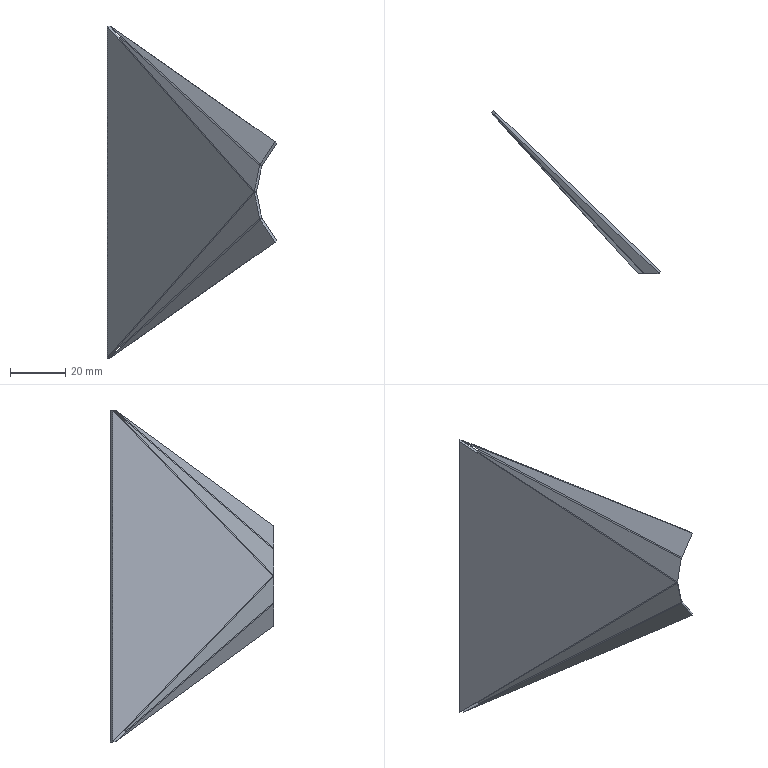Part | STEP file | JBJ-P-1003-09 | 1 solid | 42 faces | box 61.208 x 58.943 x 119.791 mm | volume 7806 mm3 | plane 32 | cylinder 8 | spline 2 | commonest cylinder face diameters 2 x4 4.4 x4
STEP:
#1=CARTESIAN_POINT('',(-30.002,-185.39,-9.425));
#2=VERTEX_POINT('',#1);
#3=CARTESIAN_POINT('',(-30.795,-186.277,-9.583));
#4=VERTEX_POINT('',#3);
#5=CARTESIAN_POINT('',(-30.002,-185.39,-9.425));
#6=DIRECTION('',(-0.6604,-0.7393,-0.1314));
#7=VECTOR('',#6,1000.);
#8=LINE('',#5,#7);
#9=EDGE_CURVE('',#2,#4,#8,.T.);
#10=ORIENTED_EDGE('',*,*,#9,.F.);
#11=CARTESIAN_POINT('',(-31.859,-185.39,-0.09366));
#12=VERTEX_POINT('',#11);
#13=CARTESIAN_POINT('',(-31.877,-185.39,0.));
#14=DIRECTION('',(0.1951,0.,-0.9808));
#15=VECTOR('',#14,1000.);
#16=LINE('',#13,#15);
#17=EDGE_CURVE('',#12,#2,#16,.T.);
#18=ORIENTED_EDGE('',*,*,#17,.F.);
#19=CARTESIAN_POINT('',(-32.651,-186.277,-0.2513));
#20=VERTEX_POINT('',#19);
#21=CARTESIAN_POINT('',(-31.859,-185.39,-0.09366));
#22=DIRECTION('',(-0.6604,-0.7393,-0.1314));
#23=VECTOR('',#22,1000.);
#24=LINE('',#21,#23);
#25=EDGE_CURVE('',#12,#20,#24,.T.);
#26=ORIENTED_EDGE('',*,*,#25,.T.);
#27=CARTESIAN_POINT('',(-32.67,-186.277,-0.1576));
#28=DIRECTION('',(0.1951,0.,-0.9808));
#29=VECTOR('',#28,1000.);
#30=LINE('',#27,#29);
#31=EDGE_CURVE('',#20,#4,#30,.T.);
#32=ORIENTED_EDGE('',*,*,#31,.T.);
#33=EDGE_LOOP('',(#10,#18,#26,#32));
#34=FACE_OUTER_BOUND('',#33,.T.);
#35=CARTESIAN_POINT('',(-31.877,-185.39,0.));
#36=DIRECTION('',(0.7251,-0.6733,0.1442));
#37=DIRECTION('',(0.1951,0.,-0.9808));
#38=AXIS2_PLACEMENT_3D('',#35,#36,#37);
#39=PLANE('',#38);
#40=ADVANCED_FACE('',(#34),#39,.T.);
#41=ORIENTED_EDGE('',*,*,#25,.F.);
#42=CARTESIAN_POINT('',(-32.113,-185.112,-0.3814));
#43=VERTEX_POINT('',#42);
#44=CARTESIAN_POINT('',(-80.984,-131.63,-55.707));
#45=DIRECTION('',(-0.5361,0.5867,-0.6069));
#46=VECTOR('',#45,1000.);
#47=LINE('',#44,#46);
#48=EDGE_CURVE('',#12,#43,#47,.T.);
#49=ORIENTED_EDGE('',*,*,#48,.T.);
#50=CARTESIAN_POINT('',(-32.905,-185.999,-0.539));
#51=VERTEX_POINT('',#50);
#52=CARTESIAN_POINT('',(-32.113,-185.112,-0.3814));
#53=DIRECTION('',(-0.6604,-0.7393,-0.1314));
#54=VECTOR('',#53,1000.);
#55=LINE('',#52,#54);
#56=EDGE_CURVE('',#43,#51,#55,.T.);
#57=ORIENTED_EDGE('',*,*,#56,.T.);
#58=CARTESIAN_POINT('',(-81.776,-132.518,-55.865));
#59=DIRECTION('',(-0.5361,0.5867,-0.6069));
#60=VECTOR('',#59,1000.);
#61=LINE('',#58,#60);
#62=EDGE_CURVE('',#20,#51,#61,.T.);
#63=ORIENTED_EDGE('',*,*,#62,.F.);
#64=EDGE_LOOP('',(#41,#49,#57,#63));
#65=FACE_OUTER_BOUND('',#64,.T.);
#66=CARTESIAN_POINT('',(-80.984,-131.63,-55.707));
#67=DIRECTION('',(0.5258,-0.3304,-0.7838));
#68=DIRECTION('',(-0.5361,0.5867,-0.6069));
#69=AXIS2_PLACEMENT_3D('',#66,#67,#68);
#70=PLANE('',#69);
#71=ADVANCED_FACE('',(#65),#70,.F.);
#72=ORIENTED_EDGE('',*,*,#56,.F.);
#73=CARTESIAN_POINT('',(-32.19,-185.047,-0.25));
#74=VERTEX_POINT('',#73);
#75=CARTESIAN_POINT('',(-31.452,-184.373,-0.25));
#76=DIRECTION('',(-0.5361,0.5867,-0.6069));
#77=DIRECTION('',(0.,0.719,0.695));
#78=AXIS2_PLACEMENT_3D('',#75,#76,#77);
#79=CIRCLE('',#78,1.);
#80=EDGE_CURVE('',#43,#74,#79,.T.);
#81=ORIENTED_EDGE('',*,*,#80,.T.);
#82=CARTESIAN_POINT('',(-33.076,-185.857,-0.25));
#83=VERTEX_POINT('',#82);
#84=CARTESIAN_POINT('',(-32.19,-185.047,-0.25));
#85=DIRECTION('',(-0.7382,-0.6746,0.));
#86=VECTOR('',#85,1000.);
#87=LINE('',#84,#86);
#88=EDGE_CURVE('',#74,#83,#87,.T.);
#89=ORIENTED_EDGE('',*,*,#88,.T.);
#90=CARTESIAN_POINT('',(-31.452,-184.373,-0.25));
#91=DIRECTION('',(-0.5361,0.5867,-0.6069));
#92=DIRECTION('',(0.,-0.719,-0.695));
#93=AXIS2_PLACEMENT_3D('',#90,#91,#92);
#94=CIRCLE('',#93,2.2);
#95=EDGE_CURVE('',#51,#83,#94,.T.);
#96=ORIENTED_EDGE('',*,*,#95,.F.);
#97=EDGE_LOOP('',(#72,#81,#89,#96));
#98=FACE_OUTER_BOUND('',#97,.T.);
#99=CARTESIAN_POINT('',(-31.452,-184.373,-0.25));
#100=DIRECTION('',(0.5361,-0.5867,0.6069));
#101=DIRECTION('',(0.,-0.719,-0.695));
#102=AXIS2_PLACEMENT_3D('',#99,#100,#101);
#103=PLANE('',#102);
#104=ADVANCED_FACE('',(#98),#103,.T.);
#105=ORIENTED_EDGE('',*,*,#88,.F.);
#106=CARTESIAN_POINT('',(-32.19,-185.047,0.25));
#107=VERTEX_POINT('',#106);
#108=CARTESIAN_POINT('',(-32.19,-185.047,0.));
#109=DIRECTION('',(0.,0.,-1.));
#110=VECTOR('',#109,1000.);
#111=LINE('',#108,#110);
#112=EDGE_CURVE('',#107,#74,#111,.T.);
#113=ORIENTED_EDGE('',*,*,#112,.F.);
#114=CARTESIAN_POINT('',(-33.076,-185.857,0.25));
#115=VERTEX_POINT('',#114);
#116=CARTESIAN_POINT('',(-32.19,-185.047,0.25));
#117=DIRECTION('',(-0.7382,-0.6746,0.));
#118=VECTOR('',#117,1000.);
#119=LINE('',#116,#118);
#120=EDGE_CURVE('',#107,#115,#119,.T.);
#121=ORIENTED_EDGE('',*,*,#120,.T.);
#122=CARTESIAN_POINT('',(-33.076,-185.857,0.));
#123=DIRECTION('',(0.,0.,-1.));
#124=VECTOR('',#123,1000.);
#125=LINE('',#122,#124);
#126=EDGE_CURVE('',#115,#83,#125,.T.);
#127=ORIENTED_EDGE('',*,*,#126,.T.);
#128=EDGE_LOOP('',(#105,#113,#121,#127));
#129=FACE_OUTER_BOUND('',#128,.T.);
#130=CARTESIAN_POINT('',(-32.19,-185.047,0.));
#131=DIRECTION('',(0.6746,-0.7382,0.));
#132=DIRECTION('',(0.,0.,-1.));
#133=AXIS2_PLACEMENT_3D('',#130,#131,#132);
#134=PLANE('',#133);
#135=ADVANCED_FACE('',(#129),#134,.T.);
#136=ORIENTED_EDGE('',*,*,#120,.F.);
#137=CARTESIAN_POINT('',(-32.113,-185.112,0.3814));
#138=VERTEX_POINT('',#137);
#139=CARTESIAN_POINT('',(-31.452,-184.373,0.25));
#140=DIRECTION('',(-0.5361,0.5867,0.6069));
#141=DIRECTION('',(0.,-0.719,0.695));
#142=AXIS2_PLACEMENT_3D('',#139,#140,#141);
#143=CIRCLE('',#142,1.);
#144=EDGE_CURVE('',#107,#138,#143,.T.);
#145=ORIENTED_EDGE('',*,*,#144,.T.);
#146=CARTESIAN_POINT('',(-32.905,-185.999,0.539));
#147=VERTEX_POINT('',#146);
#148=CARTESIAN_POINT('',(-32.113,-185.112,0.3814));
#149=DIRECTION('',(-0.6604,-0.7393,0.1314));
#150=VECTOR('',#149,1000.);
#151=LINE('',#148,#150);
#152=EDGE_CURVE('',#138,#147,#151,.T.);
#153=ORIENTED_EDGE('',*,*,#152,.T.);
#154=CARTESIAN_POINT('',(-31.452,-184.373,0.25));
#155=DIRECTION('',(-0.5361,0.5867,0.6069));
#156=DIRECTION('',(0.,0.719,-0.695));
#157=AXIS2_PLACEMENT_3D('',#154,#155,#156);
#158=CIRCLE('',#157,2.2);
#159=EDGE_CURVE('',#115,#147,#158,.T.);
#160=ORIENTED_EDGE('',*,*,#159,.F.);
#161=EDGE_LOOP('',(#136,#145,#153,#160));
#162=FACE_OUTER_BOUND('',#161,.T.);
#163=CARTESIAN_POINT('',(-31.452,-184.373,0.25));
#164=DIRECTION('',(0.5361,-0.5867,-0.6069));
#165=DIRECTION('',(0.,0.719,-0.695));
#166=AXIS2_PLACEMENT_3D('',#163,#164,#165);
#167=PLANE('',#166);
#168=ADVANCED_FACE('',(#162),#167,.T.);
#169=ORIENTED_EDGE('',*,*,#152,.F.);
#170=CARTESIAN_POINT('',(-31.859,-185.39,0.09367));
#171=VERTEX_POINT('',#170);
#172=CARTESIAN_POINT('',(-80.984,-131.63,55.707));
#173=DIRECTION('',(0.5361,-0.5867,-0.6069));
#174=VECTOR('',#173,1000.);
#175=LINE('',#172,#174);
#176=EDGE_CURVE('',#138,#171,#175,.T.);
#177=ORIENTED_EDGE('',*,*,#176,.T.);
#178=CARTESIAN_POINT('',(-32.651,-186.277,0.2513));
#179=VERTEX_POINT('',#178);
#180=CARTESIAN_POINT('',(-31.859,-185.39,0.09367));
#181=DIRECTION('',(-0.6604,-0.7393,0.1314));
#182=VECTOR('',#181,1000.);
#183=LINE('',#180,#182);
#184=EDGE_CURVE('',#171,#179,#183,.T.);
#185=ORIENTED_EDGE('',*,*,#184,.T.);
#186=CARTESIAN_POINT('',(-81.776,-132.518,55.865));
#187=DIRECTION('',(0.5361,-0.5867,-0.6069));
#188=VECTOR('',#187,1000.);
#189=LINE('',#186,#188);
#190=EDGE_CURVE('',#147,#179,#189,.T.);
#191=ORIENTED_EDGE('',*,*,#190,.F.);
#192=EDGE_LOOP('',(#169,#177,#185,#191));
#193=FACE_OUTER_BOUND('',#192,.T.);
#194=CARTESIAN_POINT('',(-80.984,-131.63,55.707));
#195=DIRECTION('',(-0.5258,0.3304,-0.7838));
#196=DIRECTION('',(0.5361,-0.5867,-0.6069));
#197=AXIS2_PLACEMENT_3D('',#194,#195,#196);
#198=PLANE('',#197);
#199=ADVANCED_FACE('',(#193),#198,.T.);
#200=ORIENTED_EDGE('',*,*,#184,.F.);
#201=CARTESIAN_POINT('',(-30.002,-185.39,9.425));
#202=VERTEX_POINT('',#201);
#203=CARTESIAN_POINT('',(-29.974,-185.39,9.567));
#204=DIRECTION('',(-0.1951,0.,-0.9808));
#205=VECTOR('',#204,1000.);
#206=LINE('',#203,#205);
#207=EDGE_CURVE('',#202,#171,#206,.T.);
#208=ORIENTED_EDGE('',*,*,#207,.F.);
#209=CARTESIAN_POINT('',(-30.795,-186.277,9.583));
#210=VERTEX_POINT('',#209);
#211=CARTESIAN_POINT('',(-30.002,-185.39,9.425));
#212=DIRECTION('',(-0.6604,-0.7393,0.1314));
#213=VECTOR('',#212,1000.);
#214=LINE('',#211,#213);
#215=EDGE_CURVE('',#202,#210,#214,.T.);
#216=ORIENTED_EDGE('',*,*,#215,.T.);
#217=CARTESIAN_POINT('',(-30.766,-186.277,9.725));
#218=DIRECTION('',(-0.1951,0.,-0.9808));
#219=VECTOR('',#218,1000.);
#220=LINE('',#217,#219);
#221=EDGE_CURVE('',#210,#179,#220,.T.);
#222=ORIENTED_EDGE('',*,*,#221,.T.);
#223=EDGE_LOOP('',(#200,#208,#216,#222));
#224=FACE_OUTER_BOUND('',#223,.T.);
#225=CARTESIAN_POINT('',(-29.974,-185.39,9.567));
#226=DIRECTION('',(-0.7251,0.6733,0.1442));
#227=DIRECTION('',(-0.1951,0.,-0.9808));
#228=AXIS2_PLACEMENT_3D('',#225,#226,#227);
#229=PLANE('',#228);
#230=ADVANCED_FACE('',(#224),#229,.F.);
#231=ORIENTED_EDGE('',*,*,#215,.F.);
#232=CARTESIAN_POINT('',(-29.9,-185.39,9.678));
#233=VERTEX_POINT('',#232);
#234=CARTESIAN_POINT('',(-30.002,-185.39,9.425));
#235=CARTESIAN_POINT('',(-29.983,-185.39,9.52));
#236=CARTESIAN_POINT('',(-29.949,-185.39,9.605));
#237=CARTESIAN_POINT('',(-29.9,-185.39,9.678));
#238=(BOUNDED_CURVE()B_SPLINE_CURVE(3,(#234,#235,#236,#237),.UNSPECIFIED.,.F.,.F.)B_SPLINE_CURVE_WITH_KNOTS((4,4),(5.926,6.188),.UNSPECIFIED.)CURVE()GEOMETRIC_REPRESENTATION_ITEM()RATIONAL_B_SPLINE_CURVE((1.,0.9943,0.9943,1.))REPRESENTATION_ITEM(''));
#239=EDGE_CURVE('',#202,#233,#238,.T.);
#240=ORIENTED_EDGE('',*,*,#239,.T.);
#241=CARTESIAN_POINT('',(-30.517,-186.333,10.09));
#242=VERTEX_POINT('',#241);
#243=CARTESIAN_POINT('',(-29.9,-185.39,9.678));
#244=DIRECTION('',(-0.5143,-0.7857,0.3437));
#245=VECTOR('',#244,1000.);
#246=LINE('',#243,#245);
#247=EDGE_CURVE('',#233,#242,#246,.T.);
#248=ORIENTED_EDGE('',*,*,#247,.T.);
#249=CARTESIAN_POINT('',(-30.795,-186.277,9.583));
#250=CARTESIAN_POINT('',(-30.726,-186.306,9.765));
#251=CARTESIAN_POINT('',(-30.633,-186.325,9.936));
#252=CARTESIAN_POINT('',(-30.517,-186.333,10.09));
#253=(BOUNDED_CURVE()B_SPLINE_CURVE(3,(#249,#250,#251,#252),.UNSPECIFIED.,.F.,.F.)B_SPLINE_CURVE_WITH_KNOTS((4,4),(5.926,6.188),.UNSPECIFIED.)CURVE()GEOMETRIC_REPRESENTATION_ITEM()RATIONAL_B_SPLINE_CURVE((1.,0.9943,0.9943,1.))REPRESENTATION_ITEM(''));
#254=EDGE_CURVE('',#210,#242,#253,.T.);
#255=ORIENTED_EDGE('',*,*,#254,.F.);
#256=EDGE_LOOP('',(#231,#240,#248,#255));
#257=FACE_OUTER_BOUND('',#256,.T.);
#258=CARTESIAN_POINT('',(-30.384,-186.337,10.251));
#259=CARTESIAN_POINT('',(-30.203,-186.021,10.085));
#260=CARTESIAN_POINT('',(-30.022,-185.706,9.919));
#261=CARTESIAN_POINT('',(-29.841,-185.39,9.753));
#262=CARTESIAN_POINT('',(-27.407,-186.337,13.492));
#263=CARTESIAN_POINT('',(-27.768,-186.021,12.736));
#264=CARTESIAN_POINT('',(-28.128,-185.706,11.981));
#265=CARTESIAN_POINT('',(-28.488,-185.39,11.226));
#266=CARTESIAN_POINT('',(-23.923,-184.443,10.291));
#267=CARTESIAN_POINT('',(-24.646,-184.759,9.868));
#268=CARTESIAN_POINT('',(-25.368,-185.074,9.445));
#269=CARTESIAN_POINT('',(-26.09,-185.39,9.022));
#270=CARTESIAN_POINT('',(-26.9,-184.443,7.051));
#271=CARTESIAN_POINT('',(-27.081,-184.759,7.217));
#272=CARTESIAN_POINT('',(-27.262,-185.074,7.383));
#273=CARTESIAN_POINT('',(-27.443,-185.39,7.549));
#274=CARTESIAN_POINT('',(-29.877,-184.443,3.811));
#275=CARTESIAN_POINT('',(-29.516,-184.759,4.566));
#276=CARTESIAN_POINT('',(-29.156,-185.074,5.321));
#277=CARTESIAN_POINT('',(-28.796,-185.39,6.077));
#278=CARTESIAN_POINT('',(-33.361,-186.337,7.011));
#279=CARTESIAN_POINT('',(-32.638,-186.021,7.434));
#280=CARTESIAN_POINT('',(-31.916,-185.706,7.857));
#281=CARTESIAN_POINT('',(-31.194,-185.39,8.28));
#282=CARTESIAN_POINT('',(-30.384,-186.337,10.251));
#283=CARTESIAN_POINT('',(-30.203,-186.021,10.085));
#284=CARTESIAN_POINT('',(-30.022,-185.706,9.919));
#285=CARTESIAN_POINT('',(-29.841,-185.39,9.753));
#286=(BOUNDED_SURFACE()B_SPLINE_SURFACE(3,3,((#258,#259,#260,#261),(#262,#263,#264,#265),(#266,#267,#268,#269),(#270,#271,#272,#273),(#274,#275,#276,#277),(#278,#279,#280,#281),(#282,#283,#284,#285)),.UNSPECIFIED.,.T.,.F.,.T.)B_SPLINE_SURFACE_WITH_KNOTS((4,3,4),(4,4),(0.,0.5,1.),(0.,1.),.UNSPECIFIED.)GEOMETRIC_REPRESENTATION_ITEM()RATIONAL_B_SPLINE_SURFACE(((1.,1.,1.,1.),(0.3333,0.3333,0.3333,0.3333),(0.3333,0.3333,0.3333,0.3333),(1.,1.,1.,1.),(0.3333,0.3333,0.3333,0.3333),(0.3333,0.3333,0.3333,0.3333),(1.,1.,1.,1.)))REPRESENTATION_ITEM('')SURFACE());
#287=ADVANCED_FACE('',(#257),#286,.F.);
#288=ORIENTED_EDGE('',*,*,#247,.F.);
#289=CARTESIAN_POINT('',(-24.555,-185.39,17.678));
#290=VERTEX_POINT('',#289);
#291=CARTESIAN_POINT('',(-24.555,-185.39,17.678));
#292=DIRECTION('',(-0.5556,0.,-0.8315));
#293=VECTOR('',#292,1000.);
#294=LINE('',#291,#293);
#295=EDGE_CURVE('',#290,#233,#294,.T.);
#296=ORIENTED_EDGE('',*,*,#295,.F.);
#297=CARTESIAN_POINT('',(-25.172,-186.333,18.09));
#298=VERTEX_POINT('',#297);
#299=CARTESIAN_POINT('',(-24.555,-185.39,17.678));
#300=DIRECTION('',(-0.5143,-0.7857,0.3437));
#301=VECTOR('',#300,1000.);
#302=LINE('',#299,#301);
#303=EDGE_CURVE('',#290,#298,#302,.T.);
#304=ORIENTED_EDGE('',*,*,#303,.T.);
#305=CARTESIAN_POINT('',(-25.172,-186.333,18.09));
#306=DIRECTION('',(-0.5556,0.,-0.8315));
#307=VECTOR('',#306,1000.);
#308=LINE('',#305,#307);
#309=EDGE_CURVE('',#298,#242,#308,.T.);
#310=ORIENTED_EDGE('',*,*,#309,.T.);
#311=EDGE_LOOP('',(#288,#296,#304,#310));
#312=FACE_OUTER_BOUND('',#311,.T.);
#313=CARTESIAN_POINT('',(-24.555,-185.39,17.678));
#314=DIRECTION('',(-0.6533,0.6186,0.4365));
#315=DIRECTION('',(-0.5556,0.,-0.8315));
#316=AXIS2_PLACEMENT_3D('',#313,#314,#315);
#317=PLANE('',#316);
#318=ADVANCED_FACE('',(#312),#317,.F.);
#319=ORIENTED_EDGE('',*,*,#303,.F.);
#320=CARTESIAN_POINT('',(-84.054,-128.181,59.423));
#321=VERTEX_POINT('',#320);
#322=CARTESIAN_POINT('',(-84.877,-127.39,60.));
#323=DIRECTION('',(0.6433,-0.6185,-0.4513));
#324=VECTOR('',#323,1000.);
#325=LINE('',#322,#324);
#326=EDGE_CURVE('',#321,#290,#325,.T.);
#327=ORIENTED_EDGE('',*,*,#326,.F.);
#328=CARTESIAN_POINT('',(-84.672,-129.124,59.835));
#329=VERTEX_POINT('',#328);
#330=CARTESIAN_POINT('',(-84.054,-128.181,59.423));
#331=DIRECTION('',(-0.5143,-0.7857,0.3437));
#332=VECTOR('',#331,1000.);
#333=LINE('',#330,#332);
#334=EDGE_CURVE('',#321,#329,#333,.T.);
#335=ORIENTED_EDGE('',*,*,#334,.T.);
#336=CARTESIAN_POINT('',(-85.494,-128.333,60.412));
#337=DIRECTION('',(0.6433,-0.6185,-0.4513));
#338=VECTOR('',#337,1000.);
#339=LINE('',#336,#338);
#340=EDGE_CURVE('',#329,#298,#339,.T.);
#341=ORIENTED_EDGE('',*,*,#340,.T.);
#342=EDGE_LOOP('',(#319,#327,#335,#341));
#343=FACE_OUTER_BOUND('',#342,.T.);
#344=CARTESIAN_POINT('',(-84.877,-127.39,60.));
#345=DIRECTION('',(-0.5672,0.01105,-0.8235));
#346=DIRECTION('',(0.6433,-0.6185,-0.4513));
#347=AXIS2_PLACEMENT_3D('',#344,#345,#346);
#348=PLANE('',#347);
#349=ADVANCED_FACE('',(#343),#348,.F.);
#350=ORIENTED_EDGE('',*,*,#334,.F.);
#351=CARTESIAN_POINT('',(-80.181,-132.273,55.864));
#352=VERTEX_POINT('',#351);
#353=CARTESIAN_POINT('',(-82.964,-129.333,58.421));
#354=DIRECTION('',(-0.5813,0.614,0.5339));
#355=VECTOR('',#354,1000.);
#356=LINE('',#353,#355);
#357=EDGE_CURVE('',#352,#321,#356,.T.);
#358=ORIENTED_EDGE('',*,*,#357,.F.);
#359=CARTESIAN_POINT('',(-80.798,-133.216,56.277));
#360=VERTEX_POINT('',#359);
#361=CARTESIAN_POINT('',(-80.181,-132.273,55.864));
#362=DIRECTION('',(-0.5143,-0.7857,0.3437));
#363=VECTOR('',#362,1000.);
#364=LINE('',#361,#363);
#365=EDGE_CURVE('',#352,#360,#364,.T.);
#366=ORIENTED_EDGE('',*,*,#365,.T.);
#367=CARTESIAN_POINT('',(-83.581,-130.276,58.834));
#368=DIRECTION('',(-0.5813,0.614,0.5339));
#369=VECTOR('',#368,1000.);
#370=LINE('',#367,#369);
#371=EDGE_CURVE('',#360,#329,#370,.T.);
#372=ORIENTED_EDGE('',*,*,#371,.T.);
#373=EDGE_LOOP('',(#350,#358,#366,#372));
#374=FACE_OUTER_BOUND('',#373,.T.);
#375=CARTESIAN_POINT('',(-82.964,-129.333,58.421));
#376=DIRECTION('',(0.6305,-0.07486,0.7725));
#377=DIRECTION('',(-0.5813,0.614,0.5339));
#378=AXIS2_PLACEMENT_3D('',#375,#376,#377);
#379=PLANE('',#378);
#380=ADVANCED_FACE('',(#374),#379,.F.);
#381=ORIENTED_EDGE('',*,*,#365,.F.);
#382=CARTESIAN_POINT('',(-80.327,-132.227,55.652));
#383=VERTEX_POINT('',#382);
#384=CARTESIAN_POINT('',(-79.666,-131.488,55.521));
#385=DIRECTION('',(0.5813,-0.614,-0.5339));
#386=DIRECTION('',(-0.7262,-0.6875,0.));
#387=AXIS2_PLACEMENT_3D('',#384,#385,#386);
#388=CIRCLE('',#387,1.);
#389=EDGE_CURVE('',#352,#383,#388,.T.);
#390=ORIENTED_EDGE('',*,*,#389,.T.);
#391=CARTESIAN_POINT('',(-81.119,-133.114,55.81));
#392=VERTEX_POINT('',#391);
#393=CARTESIAN_POINT('',(-80.327,-132.227,55.652));
#394=DIRECTION('',(-0.6604,-0.7393,0.1314));
#395=VECTOR('',#394,1000.);
#396=LINE('',#393,#395);
#397=EDGE_CURVE('',#383,#392,#396,.T.);
#398=ORIENTED_EDGE('',*,*,#397,.T.);
#399=CARTESIAN_POINT('',(-79.666,-131.488,55.521));
#400=DIRECTION('',(0.5813,-0.614,-0.5339));
#401=DIRECTION('',(-0.7262,-0.6875,0.));
#402=AXIS2_PLACEMENT_3D('',#399,#400,#401);
#403=CIRCLE('',#402,2.2);
#404=EDGE_CURVE('',#360,#392,#403,.T.);
#405=ORIENTED_EDGE('',*,*,#404,.F.);
#406=EDGE_LOOP('',(#381,#390,#398,#405));
#407=FACE_OUTER_BOUND('',#406,.T.);
#408=CARTESIAN_POINT('',(-79.666,-131.488,55.521));
#409=DIRECTION('',(0.5813,-0.614,-0.5339));
#410=DIRECTION('',(0.7262,0.6875,0.));
#411=AXIS2_PLACEMENT_3D('',#408,#409,#410);
#412=PLANE('',#411);
#413=ADVANCED_FACE('',(#407),#412,.F.);
#414=ORIENTED_EDGE('',*,*,#397,.F.);
#415=CARTESIAN_POINT('',(-80.577,-132.075,55.247));
#416=VERTEX_POINT('',#415);
#417=CARTESIAN_POINT('',(-102.873,-118.567,19.192));
#418=DIRECTION('',(0.5011,-0.3036,0.8104));
#419=VECTOR('',#418,1000.);
#420=LINE('',#417,#419);
#421=EDGE_CURVE('',#416,#383,#420,.T.);
#422=ORIENTED_EDGE('',*,*,#421,.F.);
#423=CARTESIAN_POINT('',(-81.37,-132.963,55.404));
#424=VERTEX_POINT('',#423);
#425=CARTESIAN_POINT('',(-80.577,-132.075,55.247));
#426=DIRECTION('',(-0.6604,-0.7393,0.1314));
#427=VECTOR('',#426,1000.);
#428=LINE('',#425,#427);
#429=EDGE_CURVE('',#416,#424,#428,.T.);
#430=ORIENTED_EDGE('',*,*,#429,.T.);
#431=CARTESIAN_POINT('',(-103.665,-119.454,19.35));
#432=DIRECTION('',(0.5011,-0.3036,0.8104));
#433=VECTOR('',#432,1000.);
#434=LINE('',#431,#433);
#435=EDGE_CURVE('',#424,#392,#434,.T.);
#436=ORIENTED_EDGE('',*,*,#435,.T.);
#437=EDGE_LOOP('',(#414,#422,#430,#436));
#438=FACE_OUTER_BOUND('',#437,.T.);
#439=CARTESIAN_POINT('',(-102.873,-118.567,19.192));
#440=DIRECTION('',(0.5593,-0.601,-0.571));
#441=DIRECTION('',(0.5011,-0.3036,0.8104));
#442=AXIS2_PLACEMENT_3D('',#439,#440,#441);
#443=PLANE('',#442);
#444=ADVANCED_FACE('',(#438),#443,.F.);
#445=ORIENTED_EDGE('',*,*,#429,.F.);
#446=CARTESIAN_POINT('',(-80.655,-132.011,55.115));
#447=VERTEX_POINT('',#446);
#448=CARTESIAN_POINT('',(-79.917,-131.336,55.115));
#449=DIRECTION('',(0.5361,-0.5867,-0.6069));
#450=DIRECTION('',(0.,-0.719,0.695));
#451=AXIS2_PLACEMENT_3D('',#448,#449,#450);
#452=CIRCLE('',#451,1.);
#453=EDGE_CURVE('',#416,#447,#452,.T.);
#454=ORIENTED_EDGE('',*,*,#453,.T.);
#455=CARTESIAN_POINT('',(-81.541,-132.82,55.115));
#456=VERTEX_POINT('',#455);
#457=CARTESIAN_POINT('',(-80.655,-132.011,55.115));
#458=DIRECTION('',(-0.7382,-0.6746,0.));
#459=VECTOR('',#458,1000.);
#460=LINE('',#457,#459);
#461=EDGE_CURVE('',#447,#456,#460,.T.);
#462=ORIENTED_EDGE('',*,*,#461,.T.);
#463=CARTESIAN_POINT('',(-79.917,-131.336,55.115));
#464=DIRECTION('',(0.5361,-0.5867,-0.6069));
#465=DIRECTION('',(0.,0.719,-0.695));
#466=AXIS2_PLACEMENT_3D('',#463,#464,#465);
#467=CIRCLE('',#466,2.2);
#468=EDGE_CURVE('',#424,#456,#467,.T.);
#469=ORIENTED_EDGE('',*,*,#468,.F.);
#470=EDGE_LOOP('',(#445,#454,#462,#469));
#471=FACE_OUTER_BOUND('',#470,.T.);
#472=CARTESIAN_POINT('',(-79.917,-131.336,55.115));
#473=DIRECTION('',(0.5361,-0.5867,-0.6069));
#474=DIRECTION('',(0.,0.719,-0.695));
#475=AXIS2_PLACEMENT_3D('',#472,#473,#474);
#476=PLANE('',#475);
#477=ADVANCED_FACE('',(#471),#476,.F.);
#478=ORIENTED_EDGE('',*,*,#461,.F.);
#479=CARTESIAN_POINT('',(-84.877,-127.39,59.895));
#480=VERTEX_POINT('',#479);
#481=CARTESIAN_POINT('',(-81.062,-131.566,55.576));
#482=DIRECTION('',(0.5361,-0.5867,-0.6069));
#483=VECTOR('',#482,1000.);
#484=LINE('',#481,#483);
#485=EDGE_CURVE('',#480,#447,#484,.T.);
#486=ORIENTED_EDGE('',*,*,#485,.F.);
#487=CARTESIAN_POINT('',(-85.763,-128.199,59.895));
#488=VERTEX_POINT('',#487);
#489=CARTESIAN_POINT('',(-84.877,-127.39,59.895));
#490=DIRECTION('',(-0.7382,-0.6746,0.));
#491=VECTOR('',#490,1000.);
#492=LINE('',#489,#491);
#493=EDGE_CURVE('',#480,#488,#492,.T.);
#494=ORIENTED_EDGE('',*,*,#493,.T.);
#495=CARTESIAN_POINT('',(-81.947,-132.375,55.576));
#496=DIRECTION('',(0.5361,-0.5867,-0.6069));
#497=VECTOR('',#496,1000.);
#498=LINE('',#495,#497);
#499=EDGE_CURVE('',#488,#456,#498,.T.);
#500=ORIENTED_EDGE('',*,*,#499,.T.);
#501=EDGE_LOOP('',(#478,#486,#494,#500));
#502=FACE_OUTER_BOUND('',#501,.T.);
#503=CARTESIAN_POINT('',(-81.062,-131.566,55.576));
#504=DIRECTION('',(0.4094,-0.448,0.7948));
#505=DIRECTION('',(0.5361,-0.5867,-0.6069));
#506=AXIS2_PLACEMENT_3D('',#503,#504,#505);
#507=PLANE('',#506);
#508=ADVANCED_FACE('',(#502),#507,.T.);
#509=ORIENTED_EDGE('',*,*,#493,.F.);
#510=CARTESIAN_POINT('',(-84.877,-127.39,-59.895));
#511=VERTEX_POINT('',#510);
#512=CARTESIAN_POINT('',(-84.877,-127.39,-60.));
#513=DIRECTION('',(0.,0.,1.));
#514=VECTOR('',#513,1000.);
#515=LINE('',#512,#514);
#516=EDGE_CURVE('',#511,#480,#515,.T.);
#517=ORIENTED_EDGE('',*,*,#516,.F.);
#518=CARTESIAN_POINT('',(-85.763,-128.199,-59.895));
#519=VERTEX_POINT('',#518);
#520=CARTESIAN_POINT('',(-84.877,-127.39,-59.895));
#521=DIRECTION('',(-0.7382,-0.6746,0.));
#522=VECTOR('',#521,1000.);
#523=LINE('',#520,#522);
#524=EDGE_CURVE('',#511,#519,#523,.T.);
#525=ORIENTED_EDGE('',*,*,#524,.T.);
#526=CARTESIAN_POINT('',(-85.763,-128.199,0.));
#527=DIRECTION('',(0.,0.,1.));
#528=VECTOR('',#527,1000.);
#529=LINE('',#526,#528);
#530=EDGE_CURVE('',#519,#488,#529,.T.);
#531=ORIENTED_EDGE('',*,*,#530,.T.);
#532=EDGE_LOOP('',(#509,#517,#525,#531));
#533=FACE_OUTER_BOUND('',#532,.T.);
#534=CARTESIAN_POINT('',(-84.877,-127.39,-60.));
#535=DIRECTION('',(-0.6746,0.7382,0.));
#536=DIRECTION('',(0.,0.,1.));
#537=AXIS2_PLACEMENT_3D('',#534,#535,#536);
#538=PLANE('',#537);
#539=ADVANCED_FACE('',(#533),#538,.T.);
#540=ORIENTED_EDGE('',*,*,#524,.F.);
#541=CARTESIAN_POINT('',(-80.655,-132.011,-55.115));
#542=VERTEX_POINT('',#541);
#543=CARTESIAN_POINT('',(-81.062,-131.566,-55.576));
#544=DIRECTION('',(0.5361,-0.5867,0.6069));
#545=VECTOR('',#544,1000.);
#546=LINE('',#543,#545);
#547=EDGE_CURVE('',#511,#542,#546,.T.);
#548=ORIENTED_EDGE('',*,*,#547,.T.);
#549=CARTESIAN_POINT('',(-81.541,-132.82,-55.115));
#550=VERTEX_POINT('',#549);
#551=CARTESIAN_POINT('',(-80.655,-132.011,-55.115));
#552=DIRECTION('',(-0.7382,-0.6746,0.));
#553=VECTOR('',#552,1000.);
#554=LINE('',#551,#553);
#555=EDGE_CURVE('',#542,#550,#554,.T.);
#556=ORIENTED_EDGE('',*,*,#555,.T.);
#557=CARTESIAN_POINT('',(-81.947,-132.375,-55.576));
#558=DIRECTION('',(0.5361,-0.5867,0.6069));
#559=VECTOR('',#558,1000.);
#560=LINE('',#557,#559);
#561=EDGE_CURVE('',#519,#550,#560,.T.);
#562=ORIENTED_EDGE('',*,*,#561,.F.);
#563=EDGE_LOOP('',(#540,#548,#556,#562));
#564=FACE_OUTER_BOUND('',#563,.T.);
#565=CARTESIAN_POINT('',(-81.062,-131.566,-55.576));
#566=DIRECTION('',(-0.4094,0.448,0.7948));
#567=DIRECTION('',(0.5361,-0.5867,0.6069));
#568=AXIS2_PLACEMENT_3D('',#565,#566,#567);
#569=PLANE('',#568);
#570=ADVANCED_FACE('',(#564),#569,.F.);
#571=ORIENTED_EDGE('',*,*,#555,.F.);
#572=CARTESIAN_POINT('',(-80.577,-132.076,-55.247));
#573=VERTEX_POINT('',#572);
#574=CARTESIAN_POINT('',(-79.917,-131.336,-55.115));
#575=DIRECTION('',(0.5361,-0.5867,0.6069));
#576=DIRECTION('',(0.,0.719,0.695));
#577=AXIS2_PLACEMENT_3D('',#574,#575,#576);
#578=CIRCLE('',#577,1.);
#579=EDGE_CURVE('',#542,#573,#578,.T.);
#580=ORIENTED_EDGE('',*,*,#579,.T.);
#581=CARTESIAN_POINT('',(-81.369,-132.963,-55.404));
#582=VERTEX_POINT('',#581);
#583=CARTESIAN_POINT('',(-80.577,-132.076,-55.247));
#584=DIRECTION('',(-0.6604,-0.7393,-0.1314));
#585=VECTOR('',#584,1000.);
#586=LINE('',#583,#585);
#587=EDGE_CURVE('',#573,#582,#586,.T.);
#588=ORIENTED_EDGE('',*,*,#587,.T.);
#589=CARTESIAN_POINT('',(-79.917,-131.336,-55.115));
#590=DIRECTION('',(0.5361,-0.5867,0.6069));
#591=DIRECTION('',(0.,-0.719,-0.695));
#592=AXIS2_PLACEMENT_3D('',#589,#590,#591);
#593=CIRCLE('',#592,2.2);
#594=EDGE_CURVE('',#550,#582,#593,.T.);
#595=ORIENTED_EDGE('',*,*,#594,.F.);
#596=EDGE_LOOP('',(#571,#580,#588,#595));
#597=FACE_OUTER_BOUND('',#596,.T.);
#598=CARTESIAN_POINT('',(-79.917,-131.336,-55.115));
#599=DIRECTION('',(0.5361,-0.5867,0.6069));
#600=DIRECTION('',(0.,-0.719,-0.695));
#601=AXIS2_PLACEMENT_3D('',#598,#599,#600);
#602=PLANE('',#601);
#603=ADVANCED_FACE('',(#597),#602,.F.);
#604=ORIENTED_EDGE('',*,*,#587,.F.);
#605=CARTESIAN_POINT('',(-80.326,-132.227,-55.652));
#606=VERTEX_POINT('',#605);
#607=CARTESIAN_POINT('',(-102.873,-118.566,-19.191));
#608=DIRECTION('',(0.5011,-0.3036,-0.8104));
#609=VECTOR('',#608,1000.);
#610=LINE('',#607,#609);
#611=EDGE_CURVE('',#573,#606,#610,.T.);
#612=ORIENTED_EDGE('',*,*,#611,.T.);
#613=CARTESIAN_POINT('',(-81.119,-133.115,-55.809));
#614=VERTEX_POINT('',#613);
#615=CARTESIAN_POINT('',(-80.326,-132.227,-55.652));
#616=DIRECTION('',(-0.6604,-0.7393,-0.1314));
#617=VECTOR('',#616,1000.);
#618=LINE('',#615,#617);
#619=EDGE_CURVE('',#606,#614,#618,.T.);
#620=ORIENTED_EDGE('',*,*,#619,.T.);
#621=CARTESIAN_POINT('',(-103.666,-119.454,-19.349));
#622=DIRECTION('',(0.5011,-0.3036,-0.8104));
#623=VECTOR('',#622,1000.);
#624=LINE('',#621,#623);
#625=EDGE_CURVE('',#582,#614,#624,.T.);
#626=ORIENTED_EDGE('',*,*,#625,.F.);
#627=EDGE_LOOP('',(#604,#612,#620,#626));
#628=FACE_OUTER_BOUND('',#627,.T.);
#629=CARTESIAN_POINT('',(-102.873,-118.566,-19.191));
#630=DIRECTION('',(0.5593,-0.601,0.571));
#631=DIRECTION('',(0.5011,-0.3036,-0.8104));
#632=AXIS2_PLACEMENT_3D('',#629,#630,#631);
#633=PLANE('',#632);
#634=ADVANCED_FACE('',(#628),#633,.F.);
#635=ORIENTED_EDGE('',*,*,#619,.F.);
#636=CARTESIAN_POINT('',(-80.18,-132.274,-55.864));
#637=VERTEX_POINT('',#636);
#638=CARTESIAN_POINT('',(-79.666,-131.488,-55.52));
#639=DIRECTION('',(0.5813,-0.614,0.5339));
#640=DIRECTION('',(0.7262,0.6875,0.));
#641=AXIS2_PLACEMENT_3D('',#638,#639,#640);
#642=CIRCLE('',#641,1.);
#643=EDGE_CURVE('',#606,#637,#642,.T.);
#644=ORIENTED_EDGE('',*,*,#643,.T.);
#645=CARTESIAN_POINT('',(-80.798,-133.217,-56.276));
#646=VERTEX_POINT('',#645);
#647=CARTESIAN_POINT('',(-80.18,-132.274,-55.864));
#648=DIRECTION('',(-0.5143,-0.7857,-0.3437));
#649=VECTOR('',#648,1000.);
#650=LINE('',#647,#649);
#651=EDGE_CURVE('',#637,#646,#650,.T.);
#652=ORIENTED_EDGE('',*,*,#651,.T.);
#653=CARTESIAN_POINT('',(-79.666,-131.488,-55.52));
#654=DIRECTION('',(0.5813,-0.614,0.5339));
#655=DIRECTION('',(-0.7262,-0.6875,0.));
#656=AXIS2_PLACEMENT_3D('',#653,#654,#655);
#657=CIRCLE('',#656,2.2);
#658=EDGE_CURVE('',#614,#646,#657,.T.);
#659=ORIENTED_EDGE('',*,*,#658,.F.);
#660=EDGE_LOOP('',(#635,#644,#652,#659));
#661=FACE_OUTER_BOUND('',#660,.T.);
#662=CARTESIAN_POINT('',(-79.666,-131.488,-55.52));
#663=DIRECTION('',(-0.5813,0.614,-0.5339));
#664=DIRECTION('',(-0.7262,-0.6875,0.));
#665=AXIS2_PLACEMENT_3D('',#662,#663,#664);
#666=PLANE('',#665);
#667=ADVANCED_FACE('',(#661),#666,.T.);
#668=ORIENTED_EDGE('',*,*,#651,.F.);
#669=CARTESIAN_POINT('',(-84.055,-128.181,-59.423));
#670=VERTEX_POINT('',#669);
#671=CARTESIAN_POINT('',(-82.964,-129.333,-58.421));
#672=DIRECTION('',(0.5813,-0.614,0.5339));
#673=VECTOR('',#672,1000.);
#674=LINE('',#671,#673);
#675=EDGE_CURVE('',#670,#637,#674,.T.);
#676=ORIENTED_EDGE('',*,*,#675,.F.);
#677=CARTESIAN_POINT('',(-84.672,-129.124,-59.835));
#678=VERTEX_POINT('',#677);
#679=CARTESIAN_POINT('',(-84.055,-128.181,-59.423));
#680=DIRECTION('',(-0.5143,-0.7857,-0.3437));
#681=VECTOR('',#680,1000.);
#682=LINE('',#679,#681);
#683=EDGE_CURVE('',#670,#678,#682,.T.);
#684=ORIENTED_EDGE('',*,*,#683,.T.);
#685=CARTESIAN_POINT('',(-83.581,-130.276,-58.833));
#686=DIRECTION('',(0.5813,-0.614,0.5339));
#687=VECTOR('',#686,1000.);
#688=LINE('',#685,#687);
#689=EDGE_CURVE('',#678,#646,#688,.T.);
#690=ORIENTED_EDGE('',*,*,#689,.T.);
#691=EDGE_LOOP('',(#668,#676,#684,#690));
#692=FACE_OUTER_BOUND('',#691,.T.);
#693=CARTESIAN_POINT('',(-82.964,-129.333,-58.421));
#694=DIRECTION('',(-0.6305,0.07486,0.7725));
#695=DIRECTION('',(0.5813,-0.614,0.5339));
#696=AXIS2_PLACEMENT_3D('',#693,#694,#695);
#697=PLANE('',#696);
#698=ADVANCED_FACE('',(#692),#697,.T.);
#699=ORIENTED_EDGE('',*,*,#683,.F.);
#700=CARTESIAN_POINT('',(-24.555,-185.39,-17.678));
#701=VERTEX_POINT('',#700);
#702=CARTESIAN_POINT('',(-24.555,-185.39,-17.678));
#703=DIRECTION('',(-0.6433,0.6185,-0.4513));
#704=VECTOR('',#703,1000.);
#705=LINE('',#702,#704);
#706=EDGE_CURVE('',#701,#670,#705,.T.);
#707=ORIENTED_EDGE('',*,*,#706,.F.);
#708=CARTESIAN_POINT('',(-25.172,-186.333,-18.09));
#709=VERTEX_POINT('',#708);
#710=CARTESIAN_POINT('',(-24.555,-185.39,-17.678));
#711=DIRECTION('',(-0.5143,-0.7857,-0.3437));
#712=VECTOR('',#711,1000.);
#713=LINE('',#710,#712);
#714=EDGE_CURVE('',#701,#709,#713,.T.);
#715=ORIENTED_EDGE('',*,*,#714,.T.);
#716=CARTESIAN_POINT('',(-25.172,-186.333,-18.09));
#717=DIRECTION('',(-0.6433,0.6185,-0.4513));
#718=VECTOR('',#717,1000.);
#719=LINE('',#716,#718);
#720=EDGE_CURVE('',#709,#678,#719,.T.);
#721=ORIENTED_EDGE('',*,*,#720,.T.);
#722=EDGE_LOOP('',(#699,#707,#715,#721));
#723=FACE_OUTER_BOUND('',#722,.T.);
#724=CARTESIAN_POINT('',(-24.555,-185.39,-17.678));
#725=DIRECTION('',(0.5672,-0.01106,-0.8235));
#726=DIRECTION('',(-0.6433,0.6185,-0.4513));
#727=AXIS2_PLACEMENT_3D('',#724,#725,#726);
#728=PLANE('',#727);
#729=ADVANCED_FACE('',(#723),#728,.T.);
#730=ORIENTED_EDGE('',*,*,#714,.F.);
#731=CARTESIAN_POINT('',(-29.9,-185.39,-9.678));
#732=VERTEX_POINT('',#731);
#733=CARTESIAN_POINT('',(-29.974,-185.39,-9.567));
#734=DIRECTION('',(0.5556,0.,-0.8315));
#735=VECTOR('',#734,1000.);
#736=LINE('',#733,#735);
#737=EDGE_CURVE('',#732,#701,#736,.T.);
#738=ORIENTED_EDGE('',*,*,#737,.F.);
#739=CARTESIAN_POINT('',(-30.517,-186.333,-10.09));
#740=VERTEX_POINT('',#739);
#741=CARTESIAN_POINT('',(-29.9,-185.39,-9.678));
#742=DIRECTION('',(-0.5143,-0.7857,-0.3437));
#743=VECTOR('',#742,1000.);
#744=LINE('',#741,#743);
#745=EDGE_CURVE('',#732,#740,#744,.T.);
#746=ORIENTED_EDGE('',*,*,#745,.T.);
#747=CARTESIAN_POINT('',(-30.591,-186.333,-9.979));
#748=DIRECTION('',(0.5556,0.,-0.8315));
#749=VECTOR('',#748,1000.);
#750=LINE('',#747,#749);
#751=EDGE_CURVE('',#740,#709,#750,.T.);
#752=ORIENTED_EDGE('',*,*,#751,.T.);
#753=EDGE_LOOP('',(#730,#738,#746,#752));
#754=FACE_OUTER_BOUND('',#753,.T.);
#755=CARTESIAN_POINT('',(-29.974,-185.39,-9.567));
#756=DIRECTION('',(0.6533,-0.6186,0.4365));
#757=DIRECTION('',(0.5556,0.,-0.8315));
#758=AXIS2_PLACEMENT_3D('',#755,#756,#757);
#759=PLANE('',#758);
#760=ADVANCED_FACE('',(#754),#759,.T.);
#761=CARTESIAN_POINT('',(-29.9,-185.39,-9.678));
#762=CARTESIAN_POINT('',(-29.949,-185.39,-9.604));
#763=CARTESIAN_POINT('',(-29.984,-185.39,-9.519));
#764=CARTESIAN_POINT('',(-30.002,-185.39,-9.425));
#765=(BOUNDED_CURVE()B_SPLINE_CURVE(3,(#761,#762,#763,#764),.UNSPECIFIED.,.F.,.F.)B_SPLINE_CURVE_WITH_KNOTS((4,4),(0.09499,0.3576),.UNSPECIFIED.)CURVE()GEOMETRIC_REPRESENTATION_ITEM()RATIONAL_B_SPLINE_CURVE((1.,0.9943,0.9943,1.))REPRESENTATION_ITEM(''));
#766=EDGE_CURVE('',#732,#2,#765,.T.);
#767=ORIENTED_EDGE('',*,*,#766,.T.);
#768=ORIENTED_EDGE('',*,*,#9,.T.);
#769=CARTESIAN_POINT('',(-30.517,-186.333,-10.09));
#770=CARTESIAN_POINT('',(-30.633,-186.325,-9.935));
#771=CARTESIAN_POINT('',(-30.726,-186.306,-9.765));
#772=CARTESIAN_POINT('',(-30.795,-186.277,-9.583));
#773=(BOUNDED_CURVE()B_SPLINE_CURVE(3,(#769,#770,#771,#772),.UNSPECIFIED.,.F.,.F.)B_SPLINE_CURVE_WITH_KNOTS((4,4),(0.09499,0.3576),.UNSPECIFIED.)CURVE()GEOMETRIC_REPRESENTATION_ITEM()RATIONAL_B_SPLINE_CURVE((1.,0.9943,0.9943,1.))REPRESENTATION_ITEM(''));
#774=EDGE_CURVE('',#740,#4,#773,.T.);
#775=ORIENTED_EDGE('',*,*,#774,.F.);
#776=ORIENTED_EDGE('',*,*,#745,.F.);
#777=EDGE_LOOP('',(#767,#768,#775,#776));
#778=FACE_OUTER_BOUND('',#777,.T.);
#779=CARTESIAN_POINT('',(-30.384,-186.337,-10.251));
#780=CARTESIAN_POINT('',(-30.203,-186.021,-10.085));
#781=CARTESIAN_POINT('',(-30.022,-185.706,-9.919));
#782=CARTESIAN_POINT('',(-29.842,-185.39,-9.752));
#783=CARTESIAN_POINT('',(-33.361,-186.337,-7.011));
#784=CARTESIAN_POINT('',(-32.639,-186.021,-7.434));
#785=CARTESIAN_POINT('',(-31.917,-185.706,-7.857));
#786=CARTESIAN_POINT('',(-31.194,-185.39,-8.28));
#787=CARTESIAN_POINT('',(-29.877,-184.443,-3.81));
#788=CARTESIAN_POINT('',(-29.516,-184.759,-4.566));
#789=CARTESIAN_POINT('',(-29.156,-185.074,-5.321));
#790=CARTESIAN_POINT('',(-28.796,-185.39,-6.076));
#791=CARTESIAN_POINT('',(-26.9,-184.443,-7.051));
#792=CARTESIAN_POINT('',(-27.081,-184.759,-7.217));
#793=CARTESIAN_POINT('',(-27.262,-185.074,-7.383));
#794=CARTESIAN_POINT('',(-27.443,-185.39,-7.549));
#795=CARTESIAN_POINT('',(-23.924,-184.443,-10.291));
#796=CARTESIAN_POINT('',(-24.646,-184.759,-9.868));
#797=CARTESIAN_POINT('',(-25.368,-185.074,-9.445));
#798=CARTESIAN_POINT('',(-26.09,-185.39,-9.022));
#799=CARTESIAN_POINT('',(-27.408,-186.337,-13.491));
#800=CARTESIAN_POINT('',(-27.768,-186.021,-12.736));
#801=CARTESIAN_POINT('',(-28.128,-185.706,-11.981));
#802=CARTESIAN_POINT('',(-28.489,-185.39,-11.225));
#803=CARTESIAN_POINT('',(-30.384,-186.337,-10.251));
#804=CARTESIAN_POINT('',(-30.203,-186.021,-10.085));
#805=CARTESIAN_POINT('',(-30.022,-185.706,-9.919));
#806=CARTESIAN_POINT('',(-29.842,-185.39,-9.752));
#807=(BOUNDED_SURFACE()B_SPLINE_SURFACE(3,3,((#779,#780,#781,#782),(#783,#784,#785,#786),(#787,#788,#789,#790),(#791,#792,#793,#794),(#795,#796,#797,#798),(#799,#800,#801,#802),(#803,#804,#805,#806)),.UNSPECIFIED.,.T.,.F.,.F.)B_SPLINE_SURFACE_WITH_KNOTS((4,3,4),(4,4),(0.,0.5,1.),(0.,1.),.UNSPECIFIED.)GEOMETRIC_REPRESENTATION_ITEM()RATIONAL_B_SPLINE_SURFACE(((1.,1.,1.,1.),(0.3333,0.3333,0.3333,0.3333),(0.3333,0.3333,0.3333,0.3333),(1.,1.,1.,1.),(0.3333,0.3333,0.3333,0.3333),(0.3333,0.3333,0.3333,0.3333),(1.,1.,1.,1.)))REPRESENTATION_ITEM('')SURFACE());
#808=ADVANCED_FACE('',(#778),#807,.F.);
#809=ORIENTED_EDGE('',*,*,#751,.F.);
#810=CARTESIAN_POINT('',(-83.581,-130.276,-58.833));
#811=DIRECTION('',(-0.5813,0.614,-0.5339));
#812=VECTOR('',#811,1000.);
#813=LINE('',#810,#812);
#814=EDGE_CURVE('',#740,#646,#813,.T.);
#815=ORIENTED_EDGE('',*,*,#814,.T.);
#816=ORIENTED_EDGE('',*,*,#689,.F.);
#817=ORIENTED_EDGE('',*,*,#720,.F.);
#818=EDGE_LOOP('',(#809,#815,#816,#817));
#819=FACE_OUTER_BOUND('',#818,.T.);
#820=CARTESIAN_POINT('',(-85.159,-130.089,-56.901));
#821=DIRECTION('',(0.5143,0.7857,0.3437));
#822=DIRECTION('',(-0.8367,0.5477,0.));
#823=AXIS2_PLACEMENT_3D('',#820,#821,#822);
#824=PLANE('',#823);
#825=ADVANCED_FACE('',(#819),#824,.F.);
#826=ORIENTED_EDGE('',*,*,#221,.F.);
#827=CARTESIAN_POINT('',(-83.903,-130.174,58.366));
#828=DIRECTION('',(-0.5813,0.614,0.5339));
#829=VECTOR('',#828,1000.);
#830=LINE('',#827,#829);
#831=EDGE_CURVE('',#210,#392,#830,.T.);
#832=ORIENTED_EDGE('',*,*,#831,.T.);
#833=ORIENTED_EDGE('',*,*,#435,.F.);
#834=CARTESIAN_POINT('',(-81.776,-132.518,55.865));
#835=DIRECTION('',(0.5361,-0.5867,-0.6069));
#836=VECTOR('',#835,1000.);
#837=LINE('',#834,#836);
#838=EDGE_CURVE('',#424,#147,#837,.T.);
#839=ORIENTED_EDGE('',*,*,#838,.T.);
#840=ORIENTED_EDGE('',*,*,#190,.T.);
#841=EDGE_LOOP('',(#826,#832,#833,#839,#840));
#842=FACE_OUTER_BOUND('',#841,.T.);
#843=CARTESIAN_POINT('',(-105.212,-117.792,20.929));
#844=DIRECTION('',(-0.6604,-0.7393,0.1314));
#845=DIRECTION('',(0.7458,-0.6662,0.));
#846=AXIS2_PLACEMENT_3D('',#843,#844,#845);
#847=PLANE('',#846);
#848=ADVANCED_FACE('',(#842),#847,.T.);
#849=ORIENTED_EDGE('',*,*,#561,.T.);
#850=CARTESIAN_POINT('',(-81.947,-132.375,-55.576));
#851=DIRECTION('',(0.5361,-0.5867,0.6069));
#852=VECTOR('',#851,1000.);
#853=LINE('',#850,#852);
#854=EDGE_CURVE('',#550,#83,#853,.T.);
#855=ORIENTED_EDGE('',*,*,#854,.T.);
#856=ORIENTED_EDGE('',*,*,#126,.F.);
#857=CARTESIAN_POINT('',(-81.947,-132.375,55.576));
#858=DIRECTION('',(-0.5361,0.5867,0.6069));
#859=VECTOR('',#858,1000.);
#860=LINE('',#857,#859);
#861=EDGE_CURVE('',#115,#456,#860,.T.);
#862=ORIENTED_EDGE('',*,*,#861,.T.);
#863=ORIENTED_EDGE('',*,*,#499,.F.);
#864=ORIENTED_EDGE('',*,*,#530,.F.);
#865=EDGE_LOOP('',(#849,#855,#856,#862,#863,#864));
#866=FACE_OUTER_BOUND('',#865,.T.);
#867=CARTESIAN_POINT('',(-110.577,-101.045,0.));
#868=DIRECTION('',(0.7382,0.6746,0.));
#869=DIRECTION('',(-0.6746,0.7382,0.));
#870=AXIS2_PLACEMENT_3D('',#867,#868,#869);
#871=PLANE('',#870);
#872=ADVANCED_FACE('',(#866),#871,.F.);
#873=ORIENTED_EDGE('',*,*,#371,.F.);
#874=CARTESIAN_POINT('',(-83.581,-130.276,58.834));
#875=DIRECTION('',(0.5813,-0.614,-0.5339));
#876=VECTOR('',#875,1000.);
#877=LINE('',#874,#876);
#878=EDGE_CURVE('',#360,#242,#877,.T.);
#879=ORIENTED_EDGE('',*,*,#878,.T.);
#880=ORIENTED_EDGE('',*,*,#309,.F.);
#881=ORIENTED_EDGE('',*,*,#340,.F.);
#882=EDGE_LOOP('',(#873,#879,#880,#881));
#883=FACE_OUTER_BOUND('',#882,.T.);
#884=CARTESIAN_POINT('',(-85.158,-130.089,56.902));
#885=DIRECTION('',(-0.5143,-0.7857,0.3437));
#886=DIRECTION('',(0.8367,-0.5477,0.));
#887=AXIS2_PLACEMENT_3D('',#884,#885,#886);
#888=PLANE('',#887);
#889=ADVANCED_FACE('',(#883),#888,.T.);
#890=ORIENTED_EDGE('',*,*,#625,.T.);
#891=CARTESIAN_POINT('',(-83.902,-130.174,-58.366));
#892=DIRECTION('',(0.5813,-0.614,0.5339));
#893=VECTOR('',#892,1000.);
#894=LINE('',#891,#893);
#895=EDGE_CURVE('',#614,#4,#894,.T.);
#896=ORIENTED_EDGE('',*,*,#895,.T.);
#897=ORIENTED_EDGE('',*,*,#31,.F.);
#898=ORIENTED_EDGE('',*,*,#62,.T.);
#899=CARTESIAN_POINT('',(-81.776,-132.518,-55.865));
#900=DIRECTION('',(-0.5361,0.5867,-0.6069));
#901=VECTOR('',#900,1000.);
#902=LINE('',#899,#901);
#903=EDGE_CURVE('',#51,#582,#902,.T.);
#904=ORIENTED_EDGE('',*,*,#903,.T.);
#905=EDGE_LOOP('',(#890,#896,#897,#898,#904));
#906=FACE_OUTER_BOUND('',#905,.T.);
#907=CARTESIAN_POINT('',(-105.212,-117.792,-20.928));
#908=DIRECTION('',(0.6604,0.7393,0.1314));
#909=DIRECTION('',(-0.7458,0.6662,0.));
#910=AXIS2_PLACEMENT_3D('',#907,#908,#909);
#911=PLANE('',#910);
#912=ADVANCED_FACE('',(#906),#911,.F.);
#913=ORIENTED_EDGE('',*,*,#159,.T.);
#914=ORIENTED_EDGE('',*,*,#838,.F.);
#915=ORIENTED_EDGE('',*,*,#468,.T.);
#916=ORIENTED_EDGE('',*,*,#861,.F.);
#917=EDGE_LOOP('',(#913,#914,#915,#916));
#918=FACE_OUTER_BOUND('',#917,.T.);
#919=CARTESIAN_POINT('',(-80.323,-130.891,55.576));
#920=DIRECTION('',(0.5361,-0.5867,-0.6069));
#921=DIRECTION('',(0.,0.719,-0.695));
#922=AXIS2_PLACEMENT_3D('',#919,#920,#921);
#923=CYLINDRICAL_SURFACE('',#922,2.2);
#924=ADVANCED_FACE('',(#918),#923,.T.);
#925=ORIENTED_EDGE('',*,*,#254,.T.);
#926=ORIENTED_EDGE('',*,*,#878,.F.);
#927=ORIENTED_EDGE('',*,*,#404,.T.);
#928=ORIENTED_EDGE('',*,*,#831,.F.);
#929=EDGE_LOOP('',(#925,#926,#927,#928));
#930=FACE_OUTER_BOUND('',#929,.T.);
#931=CARTESIAN_POINT('',(-82.45,-128.547,58.077));
#932=DIRECTION('',(-0.5813,0.614,0.5339));
#933=DIRECTION('',(-0.7262,-0.6875,0.));
#934=AXIS2_PLACEMENT_3D('',#931,#932,#933);
#935=CYLINDRICAL_SURFACE('',#934,2.2);
#936=ADVANCED_FACE('',(#930),#935,.T.);
#937=ORIENTED_EDGE('',*,*,#594,.T.);
#938=ORIENTED_EDGE('',*,*,#903,.F.);
#939=ORIENTED_EDGE('',*,*,#95,.T.);
#940=ORIENTED_EDGE('',*,*,#854,.F.);
#941=EDGE_LOOP('',(#937,#938,#939,#940));
#942=FACE_OUTER_BOUND('',#941,.T.);
#943=CARTESIAN_POINT('',(-80.323,-130.891,-55.576));
#944=DIRECTION('',(0.5361,-0.5867,0.6069));
#945=DIRECTION('',(0.,-0.719,-0.695));
#946=AXIS2_PLACEMENT_3D('',#943,#944,#945);
#947=CYLINDRICAL_SURFACE('',#946,2.2);
#948=ADVANCED_FACE('',(#942),#947,.T.);
#949=ORIENTED_EDGE('',*,*,#774,.T.);
#950=ORIENTED_EDGE('',*,*,#895,.F.);
#951=ORIENTED_EDGE('',*,*,#658,.T.);
#952=ORIENTED_EDGE('',*,*,#814,.F.);
#953=EDGE_LOOP('',(#949,#950,#951,#952));
#954=FACE_OUTER_BOUND('',#953,.T.);
#955=CARTESIAN_POINT('',(-82.45,-128.547,-58.077));
#956=DIRECTION('',(-0.5813,0.614,-0.5339));
#957=DIRECTION('',(-0.7262,-0.6875,0.));
#958=AXIS2_PLACEMENT_3D('',#955,#956,#957);
#959=CYLINDRICAL_SURFACE('',#958,2.2);
#960=ADVANCED_FACE('',(#954),#959,.T.);
#961=ORIENTED_EDGE('',*,*,#737,.T.);
#962=ORIENTED_EDGE('',*,*,#706,.T.);
#963=ORIENTED_EDGE('',*,*,#675,.T.);
#964=CARTESIAN_POINT('',(-82.964,-129.333,-58.421));
#965=DIRECTION('',(-0.5813,0.614,-0.5339));
#966=VECTOR('',#965,1000.);
#967=LINE('',#964,#966);
#968=EDGE_CURVE('',#732,#637,#967,.T.);
#969=ORIENTED_EDGE('',*,*,#968,.F.);
#970=EDGE_LOOP('',(#961,#962,#963,#969));
#971=FACE_OUTER_BOUND('',#970,.T.);
#972=CARTESIAN_POINT('',(-84.541,-129.146,-56.489));
#973=DIRECTION('',(0.5143,0.7857,0.3437));
#974=DIRECTION('',(-0.8367,0.5477,0.));
#975=AXIS2_PLACEMENT_3D('',#972,#973,#974);
#976=PLANE('',#975);
#977=ADVANCED_FACE('',(#971),#976,.T.);
#978=ORIENTED_EDGE('',*,*,#207,.T.);
#979=ORIENTED_EDGE('',*,*,#176,.F.);
#980=CARTESIAN_POINT('',(-32.113,-185.112,0.3814));
#981=DIRECTION('',(0.5361,-0.5867,-0.6069));
#982=VECTOR('',#981,1000.);
#983=LINE('',#980,#982);
#984=EDGE_CURVE('',#416,#138,#983,.T.);
#985=ORIENTED_EDGE('',*,*,#984,.F.);
#986=ORIENTED_EDGE('',*,*,#421,.T.);
#987=CARTESIAN_POINT('',(-83.11,-129.287,58.209));
#988=DIRECTION('',(-0.5813,0.614,0.5339));
#989=VECTOR('',#988,1000.);
#990=LINE('',#987,#989);
#991=EDGE_CURVE('',#202,#383,#990,.T.);
#992=ORIENTED_EDGE('',*,*,#991,.F.);
#993=EDGE_LOOP('',(#978,#979,#985,#986,#992));
#994=FACE_OUTER_BOUND('',#993,.T.);
#995=CARTESIAN_POINT('',(-104.419,-116.905,20.771));
#996=DIRECTION('',(-0.6604,-0.7393,0.1314));
#997=DIRECTION('',(0.7458,-0.6662,0.));
#998=AXIS2_PLACEMENT_3D('',#995,#996,#997);
#999=PLANE('',#998);
#1000=ADVANCED_FACE('',(#994),#999,.F.);
#1001=ORIENTED_EDGE('',*,*,#547,.F.);
#1002=ORIENTED_EDGE('',*,*,#516,.T.);
#1003=ORIENTED_EDGE('',*,*,#485,.T.);
#1004=CARTESIAN_POINT('',(-80.655,-132.011,55.115));
#1005=DIRECTION('',(-0.5361,0.5867,0.6069));
#1006=VECTOR('',#1005,1000.);
#1007=LINE('',#1004,#1006);
#1008=EDGE_CURVE('',#107,#447,#1007,.T.);
#1009=ORIENTED_EDGE('',*,*,#1008,.F.);
#1010=ORIENTED_EDGE('',*,*,#112,.T.);
#1011=CARTESIAN_POINT('',(-81.062,-131.566,-55.576));
#1012=DIRECTION('',(0.5361,-0.5867,0.6069));
#1013=VECTOR('',#1012,1000.);
#1014=LINE('',#1011,#1013);
#1015=EDGE_CURVE('',#542,#74,#1014,.T.);
#1016=ORIENTED_EDGE('',*,*,#1015,.F.);
#1017=EDGE_LOOP('',(#1001,#1002,#1003,#1009,#1010,#1016));
#1018=FACE_OUTER_BOUND('',#1017,.T.);
#1019=CARTESIAN_POINT('',(-109.691,-100.235,0.));
#1020=DIRECTION('',(0.7382,0.6746,0.));
#1021=DIRECTION('',(-0.6746,0.7382,0.));
#1022=AXIS2_PLACEMENT_3D('',#1019,#1020,#1021);
#1023=PLANE('',#1022);
#1024=ADVANCED_FACE('',(#1018),#1023,.T.);
#1025=ORIENTED_EDGE('',*,*,#357,.T.);
#1026=ORIENTED_EDGE('',*,*,#326,.T.);
#1027=ORIENTED_EDGE('',*,*,#295,.T.);
#1028=CARTESIAN_POINT('',(-82.964,-129.333,58.421));
#1029=DIRECTION('',(0.5813,-0.614,-0.5339));
#1030=VECTOR('',#1029,1000.);
#1031=LINE('',#1028,#1030);
#1032=EDGE_CURVE('',#352,#233,#1031,.T.);
#1033=ORIENTED_EDGE('',*,*,#1032,.F.);
#1034=EDGE_LOOP('',(#1025,#1026,#1027,#1033));
#1035=FACE_OUTER_BOUND('',#1034,.T.);
#1036=CARTESIAN_POINT('',(-84.541,-129.146,56.489));
#1037=DIRECTION('',(-0.5143,-0.7857,0.3437));
#1038=DIRECTION('',(0.8367,-0.5477,0.));
#1039=AXIS2_PLACEMENT_3D('',#1036,#1037,#1038);
#1040=PLANE('',#1039);
#1041=ADVANCED_FACE('',(#1035),#1040,.F.);
#1042=ORIENTED_EDGE('',*,*,#611,.F.);
#1043=CARTESIAN_POINT('',(-80.984,-131.63,-55.707));
#1044=DIRECTION('',(-0.5361,0.5867,-0.6069));
#1045=VECTOR('',#1044,1000.);
#1046=LINE('',#1043,#1045);
#1047=EDGE_CURVE('',#43,#573,#1046,.T.);
#1048=ORIENTED_EDGE('',*,*,#1047,.F.);
#1049=ORIENTED_EDGE('',*,*,#48,.F.);
#1050=ORIENTED_EDGE('',*,*,#17,.T.);
#1051=CARTESIAN_POINT('',(-83.11,-129.287,-58.209));
#1052=DIRECTION('',(0.5813,-0.614,0.5339));
#1053=VECTOR('',#1052,1000.);
#1054=LINE('',#1051,#1053);
#1055=EDGE_CURVE('',#606,#2,#1054,.T.);
#1056=ORIENTED_EDGE('',*,*,#1055,.F.);
#1057=EDGE_LOOP('',(#1042,#1048,#1049,#1050,#1056));
#1058=FACE_OUTER_BOUND('',#1057,.T.);
#1059=CARTESIAN_POINT('',(-104.42,-116.904,-20.77));
#1060=DIRECTION('',(0.6604,0.7393,0.1314));
#1061=DIRECTION('',(-0.7458,0.6662,0.));
#1062=AXIS2_PLACEMENT_3D('',#1059,#1060,#1061);
#1063=PLANE('',#1062);
#1064=ADVANCED_FACE('',(#1058),#1063,.T.);
#1065=ORIENTED_EDGE('',*,*,#144,.F.);
#1066=ORIENTED_EDGE('',*,*,#1008,.T.);
#1067=ORIENTED_EDGE('',*,*,#453,.F.);
#1068=ORIENTED_EDGE('',*,*,#984,.T.);
#1069=EDGE_LOOP('',(#1065,#1066,#1067,#1068));
#1070=FACE_OUTER_BOUND('',#1069,.T.);
#1071=CARTESIAN_POINT('',(-80.323,-130.891,55.576));
#1072=DIRECTION('',(0.5361,-0.5867,-0.6069));
#1073=DIRECTION('',(0.,0.719,-0.695));
#1074=AXIS2_PLACEMENT_3D('',#1071,#1072,#1073);
#1075=CYLINDRICAL_SURFACE('',#1074,1.);
#1076=ADVANCED_FACE('',(#1070),#1075,.F.);
#1077=ORIENTED_EDGE('',*,*,#239,.F.);
#1078=ORIENTED_EDGE('',*,*,#991,.T.);
#1079=ORIENTED_EDGE('',*,*,#389,.F.);
#1080=ORIENTED_EDGE('',*,*,#1032,.T.);
#1081=EDGE_LOOP('',(#1077,#1078,#1079,#1080));
#1082=FACE_OUTER_BOUND('',#1081,.T.);
#1083=CARTESIAN_POINT('',(-82.45,-128.547,58.077));
#1084=DIRECTION('',(-0.5813,0.614,0.5339));
#1085=DIRECTION('',(-0.7262,-0.6875,0.));
#1086=AXIS2_PLACEMENT_3D('',#1083,#1084,#1085);
#1087=CYLINDRICAL_SURFACE('',#1086,1.);
#1088=ADVANCED_FACE('',(#1082),#1087,.F.);
#1089=ORIENTED_EDGE('',*,*,#579,.F.);
#1090=ORIENTED_EDGE('',*,*,#1015,.T.);
#1091=ORIENTED_EDGE('',*,*,#80,.F.);
#1092=ORIENTED_EDGE('',*,*,#1047,.T.);
#1093=EDGE_LOOP('',(#1089,#1090,#1091,#1092));
#1094=FACE_OUTER_BOUND('',#1093,.T.);
#1095=CARTESIAN_POINT('',(-80.323,-130.891,-55.576));
#1096=DIRECTION('',(0.5361,-0.5867,0.6069));
#1097=DIRECTION('',(0.,-0.719,-0.695));
#1098=AXIS2_PLACEMENT_3D('',#1095,#1096,#1097);
#1099=CYLINDRICAL_SURFACE('',#1098,1.);
#1100=ADVANCED_FACE('',(#1094),#1099,.F.);
#1101=ORIENTED_EDGE('',*,*,#766,.F.);
#1102=ORIENTED_EDGE('',*,*,#968,.T.);
#1103=ORIENTED_EDGE('',*,*,#643,.F.);
#1104=ORIENTED_EDGE('',*,*,#1055,.T.);
#1105=EDGE_LOOP('',(#1101,#1102,#1103,#1104));
#1106=FACE_OUTER_BOUND('',#1105,.T.);
#1107=CARTESIAN_POINT('',(-82.45,-128.547,-58.077));
#1108=DIRECTION('',(-0.5813,0.614,-0.5339));
#1109=DIRECTION('',(-0.7262,-0.6875,0.));
#1110=AXIS2_PLACEMENT_3D('',#1107,#1108,#1109);
#1111=CYLINDRICAL_SURFACE('',#1110,1.);
#1112=ADVANCED_FACE('',(#1106),#1111,.F.);
#1113=CLOSED_SHELL('',(#40,#71,#104,#135,#168,#199,#230,#287,#318,#349,#380,#413,#444,#477,#508,#539,#570,#603,#634,#667,#698,#729,#760,#808,#825,#848,#872,#889,#912,#924,#936,#948,#960,#977,#1000,#1024,#1041,#1064,#1076,#1088,#1100,#1112));
#1114=MANIFOLD_SOLID_BREP('',#1113);
#1115=CARTESIAN_POINT('',(0.,0.,0.));
#1116=DIRECTION('',(0.,0.,1.));
#1117=DIRECTION('',(1.,0.,0.));
#1118=AXIS2_PLACEMENT_3D('',#1115,#1116,#1117);
#1119=(LENGTH_UNIT()NAMED_UNIT(*)SI_UNIT(.MILLI.,.METRE.));
#1120=UNCERTAINTY_MEASURE_WITH_UNIT(LENGTH_MEASURE(0.00001),#1119,'','');
#1121=(NAMED_UNIT(*)PLANE_ANGLE_UNIT()SI_UNIT($,.RADIAN.));
#1122=(NAMED_UNIT(*)SI_UNIT($,.STERADIAN.)SOLID_ANGLE_UNIT());
#1123=(GEOMETRIC_REPRESENTATION_CONTEXT(3)GLOBAL_UNCERTAINTY_ASSIGNED_CONTEXT((#1120))GLOBAL_UNIT_ASSIGNED_CONTEXT((#1119,#1121,#1122))REPRESENTATION_CONTEXT('',''));
#1124=ADVANCED_BREP_SHAPE_REPRESENTATION('',(#1114,#1118),#1123);